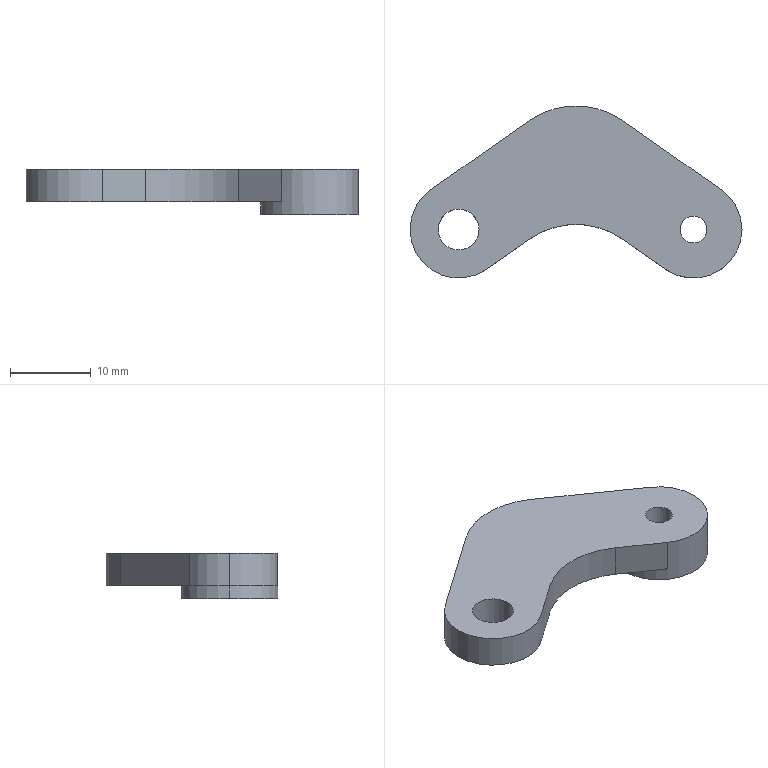Part | SolidWorks | features Attribute 3, ICE 2, Extrusion 1, Fillet 1, HoleWzd 1 | 1 solid | 17 faces | box 41 x 21.27 x 5.6 mm | volume 2205 mm3 | cylinder 10 | plane 7 | commonest cylinder face diameters 12 x4 3.3 x2 5.05 x2 20 x2
STEP:
#1=CARTESIAN_POINT('',(27.35,0.,-1.6));
#2=VERTEX_POINT('',#1);
#3=CARTESIAN_POINT('',(30.65,0.,-1.6));
#4=VERTEX_POINT('',#3);
#5=CARTESIAN_POINT('',(29.,0.,-1.6));
#6=DIRECTION('',(0.,0.,1.));
#7=DIRECTION('',(1.,0.,0.));
#8=AXIS2_PLACEMENT_3D('',#5,#6,#7);
#9=CIRCLE('',#8,1.65);
#10=EDGE_CURVE('',#2,#4,#9,.T.);
#11=ORIENTED_EDGE('',*,*,#10,.F.);
#12=CARTESIAN_POINT('',(27.35,0.,4.));
#13=VERTEX_POINT('',#12);
#14=CARTESIAN_POINT('',(27.35,0.,4.));
#15=DIRECTION('',(0.,0.,1.));
#16=VECTOR('',#15,1000.);
#17=LINE('',#14,#16);
#18=EDGE_CURVE('',#2,#13,#17,.T.);
#19=ORIENTED_EDGE('',*,*,#18,.T.);
#20=CARTESIAN_POINT('',(30.65,0.,4.));
#21=VERTEX_POINT('',#20);
#22=CARTESIAN_POINT('',(29.,0.,4.));
#23=DIRECTION('',(0.,0.,1.));
#24=DIRECTION('',(1.,0.,0.));
#25=AXIS2_PLACEMENT_3D('',#22,#23,#24);
#26=CIRCLE('',#25,1.65);
#27=EDGE_CURVE('',#13,#21,#26,.T.);
#28=ORIENTED_EDGE('',*,*,#27,.T.);
#29=CARTESIAN_POINT('',(30.65,0.,4.));
#30=DIRECTION('',(0.,0.,1.));
#31=VECTOR('',#30,1000.);
#32=LINE('',#29,#31);
#33=EDGE_CURVE('',#4,#21,#32,.T.);
#34=ORIENTED_EDGE('',*,*,#33,.F.);
#35=EDGE_LOOP('',(#11,#19,#28,#34));
#36=FACE_OUTER_BOUND('',#35,.T.);
#37=CARTESIAN_POINT('',(29.,0.,4.));
#38=DIRECTION('',(0.,0.,1.));
#39=DIRECTION('',(1.,0.,0.));
#40=AXIS2_PLACEMENT_3D('',#37,#38,#39);
#41=CYLINDRICAL_SURFACE('',#40,1.65);
#42=ADVANCED_FACE('',(#36),#41,.F.);
#43=CARTESIAN_POINT('',(-2.525,0.,0.));
#44=VERTEX_POINT('',#43);
#45=CARTESIAN_POINT('',(2.525,0.,0.));
#46=VERTEX_POINT('',#45);
#47=CARTESIAN_POINT('',(0.,0.,0.));
#48=DIRECTION('',(0.,0.,1.));
#49=DIRECTION('',(1.,0.,0.));
#50=AXIS2_PLACEMENT_3D('',#47,#48,#49);
#51=CIRCLE('',#50,2.525);
#52=EDGE_CURVE('',#44,#46,#51,.T.);
#53=ORIENTED_EDGE('',*,*,#52,.F.);
#54=CARTESIAN_POINT('',(-2.525,0.,4.));
#55=VERTEX_POINT('',#54);
#56=CARTESIAN_POINT('',(-2.525,0.,-1.));
#57=DIRECTION('',(0.,0.,1.));
#58=VECTOR('',#57,1000.);
#59=LINE('',#56,#58);
#60=EDGE_CURVE('',#44,#55,#59,.T.);
#61=ORIENTED_EDGE('',*,*,#60,.T.);
#62=CARTESIAN_POINT('',(2.525,0.,4.));
#63=VERTEX_POINT('',#62);
#64=CARTESIAN_POINT('',(0.,0.,4.));
#65=DIRECTION('',(0.,0.,1.));
#66=DIRECTION('',(1.,0.,0.));
#67=AXIS2_PLACEMENT_3D('',#64,#65,#66);
#68=CIRCLE('',#67,2.525);
#69=EDGE_CURVE('',#55,#63,#68,.T.);
#70=ORIENTED_EDGE('',*,*,#69,.T.);
#71=CARTESIAN_POINT('',(2.525,0.,-1.));
#72=DIRECTION('',(0.,0.,1.));
#73=VECTOR('',#72,1000.);
#74=LINE('',#71,#73);
#75=EDGE_CURVE('',#46,#63,#74,.T.);
#76=ORIENTED_EDGE('',*,*,#75,.F.);
#77=EDGE_LOOP('',(#53,#61,#70,#76));
#78=FACE_OUTER_BOUND('',#77,.T.);
#79=CARTESIAN_POINT('',(0.,0.,-1.));
#80=DIRECTION('',(0.,0.,1.));
#81=DIRECTION('',(1.,0.,0.));
#82=AXIS2_PLACEMENT_3D('',#79,#80,#81);
#83=CYLINDRICAL_SURFACE('',#82,2.525);
#84=ADVANCED_FACE('',(#78),#83,.F.);
#85=CARTESIAN_POINT('',(35.,0.,4.));
#86=VERTEX_POINT('',#85);
#87=CARTESIAN_POINT('',(32.441,4.915,4.));
#88=VERTEX_POINT('',#87);
#89=CARTESIAN_POINT('',(29.,0.,4.));
#90=DIRECTION('',(0.,0.,1.));
#91=DIRECTION('',(1.,0.,0.));
#92=AXIS2_PLACEMENT_3D('',#89,#90,#91);
#93=CIRCLE('',#92,6.);
#94=EDGE_CURVE('',#86,#88,#93,.T.);
#95=ORIENTED_EDGE('',*,*,#94,.F.);
#96=CARTESIAN_POINT('',(35.,0.,-1.6));
#97=VERTEX_POINT('',#96);
#98=CARTESIAN_POINT('',(35.,0.,4.));
#99=DIRECTION('',(0.,0.,-1.));
#100=VECTOR('',#99,1000.);
#101=LINE('',#98,#100);
#102=EDGE_CURVE('',#86,#97,#101,.T.);
#103=ORIENTED_EDGE('',*,*,#102,.T.);
#104=CARTESIAN_POINT('',(23.,0.,-1.6));
#105=VERTEX_POINT('',#104);
#106=CARTESIAN_POINT('',(29.,0.,-1.6));
#107=DIRECTION('',(0.,0.,-1.));
#108=DIRECTION('',(-1.,0.,0.));
#109=AXIS2_PLACEMENT_3D('',#106,#107,#108);
#110=CIRCLE('',#109,6.);
#111=EDGE_CURVE('',#105,#97,#110,.T.);
#112=ORIENTED_EDGE('',*,*,#111,.F.);
#113=CARTESIAN_POINT('',(23.,0.,0.));
#114=VERTEX_POINT('',#113);
#115=CARTESIAN_POINT('',(23.,0.,4.));
#116=DIRECTION('',(0.,0.,-1.));
#117=VECTOR('',#116,1000.);
#118=LINE('',#115,#117);
#119=EDGE_CURVE('',#114,#105,#118,.T.);
#120=ORIENTED_EDGE('',*,*,#119,.F.);
#121=CARTESIAN_POINT('',(32.441,4.915,0.));
#122=VERTEX_POINT('',#121);
#123=CARTESIAN_POINT('',(29.,0.,0.));
#124=DIRECTION('',(0.,0.,-1.));
#125=DIRECTION('',(-1.,0.,0.));
#126=AXIS2_PLACEMENT_3D('',#123,#124,#125);
#127=CIRCLE('',#126,6.);
#128=EDGE_CURVE('',#114,#122,#127,.T.);
#129=ORIENTED_EDGE('',*,*,#128,.T.);
#130=CARTESIAN_POINT('',(32.441,4.915,4.));
#131=DIRECTION('',(0.,0.,-1.));
#132=VECTOR('',#131,1000.);
#133=LINE('',#130,#132);
#134=EDGE_CURVE('',#88,#122,#133,.T.);
#135=ORIENTED_EDGE('',*,*,#134,.F.);
#136=EDGE_LOOP('',(#95,#103,#112,#120,#129,#135));
#137=FACE_OUTER_BOUND('',#136,.T.);
#138=CARTESIAN_POINT('',(29.,0.,4.));
#139=DIRECTION('',(0.,0.,-1.));
#140=DIRECTION('',(-1.,0.,0.));
#141=AXIS2_PLACEMENT_3D('',#138,#139,#140);
#142=CYLINDRICAL_SURFACE('',#141,6.);
#143=ADVANCED_FACE('',(#137),#142,.T.);
#144=CARTESIAN_POINT('',(-6.,0.,4.));
#145=VERTEX_POINT('',#144);
#146=CARTESIAN_POINT('',(3.441,-4.915,4.));
#147=VERTEX_POINT('',#146);
#148=CARTESIAN_POINT('',(0.,0.,4.));
#149=DIRECTION('',(0.,0.,1.));
#150=DIRECTION('',(1.,0.,0.));
#151=AXIS2_PLACEMENT_3D('',#148,#149,#150);
#152=CIRCLE('',#151,6.);
#153=EDGE_CURVE('',#145,#147,#152,.T.);
#154=ORIENTED_EDGE('',*,*,#153,.F.);
#155=CARTESIAN_POINT('',(-6.,0.,0.));
#156=VERTEX_POINT('',#155);
#157=CARTESIAN_POINT('',(-6.,0.,4.));
#158=DIRECTION('',(0.,0.,-1.));
#159=VECTOR('',#158,1000.);
#160=LINE('',#157,#159);
#161=EDGE_CURVE('',#145,#156,#160,.T.);
#162=ORIENTED_EDGE('',*,*,#161,.T.);
#163=CARTESIAN_POINT('',(3.441,-4.915,0.));
#164=VERTEX_POINT('',#163);
#165=CARTESIAN_POINT('',(0.,0.,0.));
#166=DIRECTION('',(0.,0.,1.));
#167=DIRECTION('',(1.,0.,0.));
#168=AXIS2_PLACEMENT_3D('',#165,#166,#167);
#169=CIRCLE('',#168,6.);
#170=EDGE_CURVE('',#156,#164,#169,.T.);
#171=ORIENTED_EDGE('',*,*,#170,.T.);
#172=CARTESIAN_POINT('',(3.441,-4.915,4.));
#173=DIRECTION('',(0.,0.,-1.));
#174=VECTOR('',#173,1000.);
#175=LINE('',#172,#174);
#176=EDGE_CURVE('',#147,#164,#175,.T.);
#177=ORIENTED_EDGE('',*,*,#176,.F.);
#178=EDGE_LOOP('',(#154,#162,#171,#177));
#179=FACE_OUTER_BOUND('',#178,.T.);
#180=CARTESIAN_POINT('',(0.,0.,4.));
#181=DIRECTION('',(0.,0.,-1.));
#182=DIRECTION('',(-1.,0.,0.));
#183=AXIS2_PLACEMENT_3D('',#180,#181,#182);
#184=CYLINDRICAL_SURFACE('',#183,6.);
#185=ADVANCED_FACE('',(#179),#184,.T.);
#186=ORIENTED_EDGE('',*,*,#161,.F.);
#187=CARTESIAN_POINT('',(-3.441,4.915,4.));
#188=VERTEX_POINT('',#187);
#189=CARTESIAN_POINT('',(0.,0.,4.));
#190=DIRECTION('',(0.,0.,1.));
#191=DIRECTION('',(1.,0.,0.));
#192=AXIS2_PLACEMENT_3D('',#189,#190,#191);
#193=CIRCLE('',#192,6.);
#194=EDGE_CURVE('',#188,#145,#193,.T.);
#195=ORIENTED_EDGE('',*,*,#194,.F.);
#196=CARTESIAN_POINT('',(-3.441,4.915,0.));
#197=VERTEX_POINT('',#196);
#198=CARTESIAN_POINT('',(-3.441,4.915,4.));
#199=DIRECTION('',(0.,0.,-1.));
#200=VECTOR('',#199,1000.);
#201=LINE('',#198,#200);
#202=EDGE_CURVE('',#188,#197,#201,.T.);
#203=ORIENTED_EDGE('',*,*,#202,.T.);
#204=CARTESIAN_POINT('',(0.,0.,0.));
#205=DIRECTION('',(0.,0.,1.));
#206=DIRECTION('',(1.,0.,0.));
#207=AXIS2_PLACEMENT_3D('',#204,#205,#206);
#208=CIRCLE('',#207,6.);
#209=EDGE_CURVE('',#197,#156,#208,.T.);
#210=ORIENTED_EDGE('',*,*,#209,.T.);
#211=EDGE_LOOP('',(#186,#195,#203,#210));
#212=FACE_OUTER_BOUND('',#211,.T.);
#213=CARTESIAN_POINT('',(0.,0.,4.));
#214=DIRECTION('',(0.,0.,-1.));
#215=DIRECTION('',(-1.,0.,0.));
#216=AXIS2_PLACEMENT_3D('',#213,#214,#215);
#217=CYLINDRICAL_SURFACE('',#216,6.);
#218=ADVANCED_FACE('',(#212),#217,.T.);
#219=CARTESIAN_POINT('',(8.764,-1.188,0.));
#220=VERTEX_POINT('',#219);
#221=CARTESIAN_POINT('',(3.441,-4.915,0.));
#222=DIRECTION('',(0.8192,0.5736,0.));
#223=VECTOR('',#222,1000.);
#224=LINE('',#221,#223);
#225=EDGE_CURVE('',#164,#220,#224,.T.);
#226=ORIENTED_EDGE('',*,*,#225,.T.);
#227=CARTESIAN_POINT('',(8.764,-1.188,4.));
#228=VERTEX_POINT('',#227);
#229=CARTESIAN_POINT('',(8.764,-1.188,4.));
#230=DIRECTION('',(0.,0.,1.));
#231=VECTOR('',#230,1000.);
#232=LINE('',#229,#231);
#233=EDGE_CURVE('',#220,#228,#232,.T.);
#234=ORIENTED_EDGE('',*,*,#233,.T.);
#235=CARTESIAN_POINT('',(3.441,-4.915,4.));
#236=DIRECTION('',(0.8192,0.5736,0.));
#237=VECTOR('',#236,1000.);
#238=LINE('',#235,#237);
#239=EDGE_CURVE('',#147,#228,#238,.T.);
#240=ORIENTED_EDGE('',*,*,#239,.F.);
#241=ORIENTED_EDGE('',*,*,#176,.T.);
#242=EDGE_LOOP('',(#226,#234,#240,#241));
#243=FACE_OUTER_BOUND('',#242,.T.);
#244=CARTESIAN_POINT('',(3.441,-4.915,4.));
#245=DIRECTION('',(-0.5736,0.8192,0.));
#246=DIRECTION('',(-0.8192,-0.5736,0.));
#247=AXIS2_PLACEMENT_3D('',#244,#245,#246);
#248=PLANE('',#247);
#249=ADVANCED_FACE('',(#243),#248,.F.);
#250=CARTESIAN_POINT('',(20.236,-1.188,4.));
#251=VERTEX_POINT('',#250);
#252=CARTESIAN_POINT('',(25.559,-4.915,4.));
#253=VERTEX_POINT('',#252);
#254=CARTESIAN_POINT('',(14.5,2.828,4.));
#255=DIRECTION('',(0.8192,-0.5736,0.));
#256=VECTOR('',#255,1000.);
#257=LINE('',#254,#256);
#258=EDGE_CURVE('',#251,#253,#257,.T.);
#259=ORIENTED_EDGE('',*,*,#258,.F.);
#260=CARTESIAN_POINT('',(20.236,-1.188,0.));
#261=VERTEX_POINT('',#260);
#262=CARTESIAN_POINT('',(20.236,-1.188,0.));
#263=DIRECTION('',(0.,0.,-1.));
#264=VECTOR('',#263,1000.);
#265=LINE('',#262,#264);
#266=EDGE_CURVE('',#251,#261,#265,.T.);
#267=ORIENTED_EDGE('',*,*,#266,.T.);
#268=CARTESIAN_POINT('',(25.559,-4.915,0.));
#269=VERTEX_POINT('',#268);
#270=CARTESIAN_POINT('',(14.5,2.828,0.));
#271=DIRECTION('',(0.8192,-0.5736,0.));
#272=VECTOR('',#271,1000.);
#273=LINE('',#270,#272);
#274=EDGE_CURVE('',#261,#269,#273,.T.);
#275=ORIENTED_EDGE('',*,*,#274,.T.);
#276=CARTESIAN_POINT('',(25.559,-4.915,4.));
#277=DIRECTION('',(0.,0.,-1.));
#278=VECTOR('',#277,1000.);
#279=LINE('',#276,#278);
#280=EDGE_CURVE('',#253,#269,#279,.T.);
#281=ORIENTED_EDGE('',*,*,#280,.F.);
#282=EDGE_LOOP('',(#259,#267,#275,#281));
#283=FACE_OUTER_BOUND('',#282,.T.);
#284=CARTESIAN_POINT('',(14.5,2.828,4.));
#285=DIRECTION('',(0.5736,0.8192,0.));
#286=DIRECTION('',(-0.8192,0.5736,0.));
#287=AXIS2_PLACEMENT_3D('',#284,#285,#286);
#288=PLANE('',#287);
#289=ADVANCED_FACE('',(#283),#288,.F.);
#290=ORIENTED_EDGE('',*,*,#102,.F.);
#291=CARTESIAN_POINT('',(29.,0.,4.));
#292=DIRECTION('',(0.,0.,1.));
#293=DIRECTION('',(1.,0.,0.));
#294=AXIS2_PLACEMENT_3D('',#291,#292,#293);
#295=CIRCLE('',#294,6.);
#296=EDGE_CURVE('',#253,#86,#295,.T.);
#297=ORIENTED_EDGE('',*,*,#296,.F.);
#298=ORIENTED_EDGE('',*,*,#280,.T.);
#299=CARTESIAN_POINT('',(29.,0.,0.));
#300=DIRECTION('',(0.,0.,-1.));
#301=DIRECTION('',(-1.,0.,0.));
#302=AXIS2_PLACEMENT_3D('',#299,#300,#301);
#303=CIRCLE('',#302,6.);
#304=EDGE_CURVE('',#269,#114,#303,.T.);
#305=ORIENTED_EDGE('',*,*,#304,.T.);
#306=ORIENTED_EDGE('',*,*,#119,.T.);
#307=CARTESIAN_POINT('',(29.,0.,-1.6));
#308=DIRECTION('',(0.,0.,-1.));
#309=DIRECTION('',(-1.,0.,0.));
#310=AXIS2_PLACEMENT_3D('',#307,#308,#309);
#311=CIRCLE('',#310,6.);
#312=EDGE_CURVE('',#97,#105,#311,.T.);
#313=ORIENTED_EDGE('',*,*,#312,.F.);
#314=EDGE_LOOP('',(#290,#297,#298,#305,#306,#313));
#315=FACE_OUTER_BOUND('',#314,.T.);
#316=CARTESIAN_POINT('',(29.,0.,4.));
#317=DIRECTION('',(0.,0.,-1.));
#318=DIRECTION('',(-1.,0.,0.));
#319=AXIS2_PLACEMENT_3D('',#316,#317,#318);
#320=CYLINDRICAL_SURFACE('',#319,6.);
#321=ADVANCED_FACE('',(#315),#320,.T.);
#322=CARTESIAN_POINT('',(20.236,13.461,0.));
#323=VERTEX_POINT('',#322);
#324=CARTESIAN_POINT('',(14.5,17.478,0.));
#325=DIRECTION('',(-0.8192,0.5736,0.));
#326=VECTOR('',#325,1000.);
#327=LINE('',#324,#326);
#328=EDGE_CURVE('',#122,#323,#327,.T.);
#329=ORIENTED_EDGE('',*,*,#328,.T.);
#330=CARTESIAN_POINT('',(20.236,13.461,4.));
#331=VERTEX_POINT('',#330);
#332=CARTESIAN_POINT('',(20.236,13.461,4.));
#333=DIRECTION('',(0.,0.,1.));
#334=VECTOR('',#333,1000.);
#335=LINE('',#332,#334);
#336=EDGE_CURVE('',#323,#331,#335,.T.);
#337=ORIENTED_EDGE('',*,*,#336,.T.);
#338=CARTESIAN_POINT('',(14.5,17.478,4.));
#339=DIRECTION('',(-0.8192,0.5736,0.));
#340=VECTOR('',#339,1000.);
#341=LINE('',#338,#340);
#342=EDGE_CURVE('',#88,#331,#341,.T.);
#343=ORIENTED_EDGE('',*,*,#342,.F.);
#344=ORIENTED_EDGE('',*,*,#134,.T.);
#345=EDGE_LOOP('',(#329,#337,#343,#344));
#346=FACE_OUTER_BOUND('',#345,.T.);
#347=CARTESIAN_POINT('',(14.5,17.478,4.));
#348=DIRECTION('',(-0.5736,-0.8192,0.));
#349=DIRECTION('',(0.8192,-0.5736,0.));
#350=AXIS2_PLACEMENT_3D('',#347,#348,#349);
#351=PLANE('',#350);
#352=ADVANCED_FACE('',(#346),#351,.F.);
#353=CARTESIAN_POINT('',(8.764,13.461,4.));
#354=VERTEX_POINT('',#353);
#355=CARTESIAN_POINT('',(-3.441,4.915,4.));
#356=DIRECTION('',(-0.8192,-0.5736,0.));
#357=VECTOR('',#356,1000.);
#358=LINE('',#355,#357);
#359=EDGE_CURVE('',#354,#188,#358,.T.);
#360=ORIENTED_EDGE('',*,*,#359,.F.);
#361=CARTESIAN_POINT('',(8.764,13.461,0.));
#362=VERTEX_POINT('',#361);
#363=CARTESIAN_POINT('',(8.764,13.461,4.));
#364=DIRECTION('',(0.,0.,-1.));
#365=VECTOR('',#364,1000.);
#366=LINE('',#363,#365);
#367=EDGE_CURVE('',#354,#362,#366,.T.);
#368=ORIENTED_EDGE('',*,*,#367,.T.);
#369=CARTESIAN_POINT('',(-3.441,4.915,0.));
#370=DIRECTION('',(-0.8192,-0.5736,0.));
#371=VECTOR('',#370,1000.);
#372=LINE('',#369,#371);
#373=EDGE_CURVE('',#362,#197,#372,.T.);
#374=ORIENTED_EDGE('',*,*,#373,.T.);
#375=ORIENTED_EDGE('',*,*,#202,.F.);
#376=EDGE_LOOP('',(#360,#368,#374,#375));
#377=FACE_OUTER_BOUND('',#376,.T.);
#378=CARTESIAN_POINT('',(-3.441,4.915,4.));
#379=DIRECTION('',(0.5736,-0.8192,0.));
#380=DIRECTION('',(0.8192,0.5736,0.));
#381=AXIS2_PLACEMENT_3D('',#378,#379,#380);
#382=PLANE('',#381);
#383=ADVANCED_FACE('',(#377),#382,.F.);
#384=CARTESIAN_POINT('',(29.,0.,4.));
#385=DIRECTION('',(0.,0.,1.));
#386=DIRECTION('',(1.,0.,0.));
#387=AXIS2_PLACEMENT_3D('',#384,#385,#386);
#388=CIRCLE('',#387,1.65);
#389=EDGE_CURVE('',#21,#13,#388,.T.);
#390=ORIENTED_EDGE('',*,*,#389,.F.);
#391=ORIENTED_EDGE('',*,*,#27,.F.);
#392=EDGE_LOOP('',(#390,#391));
#393=FACE_BOUND('',#392,.T.);
#394=CARTESIAN_POINT('',(0.,0.,4.));
#395=DIRECTION('',(0.,0.,1.));
#396=DIRECTION('',(1.,0.,0.));
#397=AXIS2_PLACEMENT_3D('',#394,#395,#396);
#398=CIRCLE('',#397,2.525);
#399=EDGE_CURVE('',#63,#55,#398,.T.);
#400=ORIENTED_EDGE('',*,*,#399,.F.);
#401=ORIENTED_EDGE('',*,*,#69,.F.);
#402=EDGE_LOOP('',(#400,#401));
#403=FACE_BOUND('',#402,.T.);
#404=ORIENTED_EDGE('',*,*,#342,.T.);
#405=CARTESIAN_POINT('',(14.5,5.27,4.));
#406=DIRECTION('',(0.,0.,1.));
#407=DIRECTION('',(1.,0.,0.));
#408=AXIS2_PLACEMENT_3D('',#405,#406,#407);
#409=CIRCLE('',#408,10.);
#410=EDGE_CURVE('',#331,#354,#409,.T.);
#411=ORIENTED_EDGE('',*,*,#410,.T.);
#412=ORIENTED_EDGE('',*,*,#359,.T.);
#413=ORIENTED_EDGE('',*,*,#194,.T.);
#414=ORIENTED_EDGE('',*,*,#153,.T.);
#415=ORIENTED_EDGE('',*,*,#239,.T.);
#416=CARTESIAN_POINT('',(14.5,-9.379,4.));
#417=DIRECTION('',(0.,0.,-1.));
#418=DIRECTION('',(1.,0.,0.));
#419=AXIS2_PLACEMENT_3D('',#416,#417,#418);
#420=CIRCLE('',#419,10.);
#421=EDGE_CURVE('',#228,#251,#420,.T.);
#422=ORIENTED_EDGE('',*,*,#421,.T.);
#423=ORIENTED_EDGE('',*,*,#258,.T.);
#424=ORIENTED_EDGE('',*,*,#296,.T.);
#425=ORIENTED_EDGE('',*,*,#94,.T.);
#426=EDGE_LOOP('',(#404,#411,#412,#413,#414,#415,#422,#423,#424,#425));
#427=FACE_OUTER_BOUND('',#426,.T.);
#428=CARTESIAN_POINT('',(0.,0.,4.));
#429=DIRECTION('',(0.,0.,1.));
#430=DIRECTION('',(1.,0.,0.));
#431=AXIS2_PLACEMENT_3D('',#428,#429,#430);
#432=PLANE('',#431);
#433=ADVANCED_FACE('',(#393,#403,#427),#432,.T.);
#434=ORIENTED_EDGE('',*,*,#373,.F.);
#435=CARTESIAN_POINT('',(14.5,5.27,0.));
#436=DIRECTION('',(0.,0.,-1.));
#437=DIRECTION('',(1.,0.,0.));
#438=AXIS2_PLACEMENT_3D('',#435,#436,#437);
#439=CIRCLE('',#438,10.);
#440=EDGE_CURVE('',#362,#323,#439,.T.);
#441=ORIENTED_EDGE('',*,*,#440,.T.);
#442=ORIENTED_EDGE('',*,*,#328,.F.);
#443=ORIENTED_EDGE('',*,*,#128,.F.);
#444=ORIENTED_EDGE('',*,*,#304,.F.);
#445=ORIENTED_EDGE('',*,*,#274,.F.);
#446=CARTESIAN_POINT('',(14.5,-9.379,0.));
#447=DIRECTION('',(0.,0.,1.));
#448=DIRECTION('',(1.,0.,0.));
#449=AXIS2_PLACEMENT_3D('',#446,#447,#448);
#450=CIRCLE('',#449,10.);
#451=EDGE_CURVE('',#261,#220,#450,.T.);
#452=ORIENTED_EDGE('',*,*,#451,.T.);
#453=ORIENTED_EDGE('',*,*,#225,.F.);
#454=ORIENTED_EDGE('',*,*,#170,.F.);
#455=ORIENTED_EDGE('',*,*,#209,.F.);
#456=EDGE_LOOP('',(#434,#441,#442,#443,#444,#445,#452,#453,#454,#455));
#457=FACE_OUTER_BOUND('',#456,.T.);
#458=CARTESIAN_POINT('',(0.,0.,0.));
#459=DIRECTION('',(0.,0.,1.));
#460=DIRECTION('',(1.,0.,0.));
#461=AXIS2_PLACEMENT_3D('',#458,#459,#460);
#462=CIRCLE('',#461,2.525);
#463=EDGE_CURVE('',#46,#44,#462,.T.);
#464=ORIENTED_EDGE('',*,*,#463,.T.);
#465=ORIENTED_EDGE('',*,*,#52,.T.);
#466=EDGE_LOOP('',(#464,#465));
#467=FACE_BOUND('',#466,.T.);
#468=CARTESIAN_POINT('',(0.,0.,0.));
#469=DIRECTION('',(0.,0.,1.));
#470=DIRECTION('',(1.,0.,0.));
#471=AXIS2_PLACEMENT_3D('',#468,#469,#470);
#472=PLANE('',#471);
#473=ADVANCED_FACE('',(#457,#467),#472,.F.);
#474=ORIENTED_EDGE('',*,*,#60,.F.);
#475=ORIENTED_EDGE('',*,*,#463,.F.);
#476=ORIENTED_EDGE('',*,*,#75,.T.);
#477=ORIENTED_EDGE('',*,*,#399,.T.);
#478=EDGE_LOOP('',(#474,#475,#476,#477));
#479=FACE_OUTER_BOUND('',#478,.T.);
#480=CARTESIAN_POINT('',(0.,0.,-1.));
#481=DIRECTION('',(0.,0.,1.));
#482=DIRECTION('',(1.,0.,0.));
#483=AXIS2_PLACEMENT_3D('',#480,#481,#482);
#484=CYLINDRICAL_SURFACE('',#483,2.525);
#485=ADVANCED_FACE('',(#479),#484,.F.);
#486=CARTESIAN_POINT('',(29.,0.,-1.6));
#487=DIRECTION('',(0.,0.,1.));
#488=DIRECTION('',(1.,0.,0.));
#489=AXIS2_PLACEMENT_3D('',#486,#487,#488);
#490=CIRCLE('',#489,1.65);
#491=EDGE_CURVE('',#4,#2,#490,.T.);
#492=ORIENTED_EDGE('',*,*,#491,.T.);
#493=ORIENTED_EDGE('',*,*,#10,.T.);
#494=EDGE_LOOP('',(#492,#493));
#495=FACE_BOUND('',#494,.T.);
#496=ORIENTED_EDGE('',*,*,#111,.T.);
#497=ORIENTED_EDGE('',*,*,#312,.T.);
#498=EDGE_LOOP('',(#496,#497));
#499=FACE_OUTER_BOUND('',#498,.T.);
#500=CARTESIAN_POINT('',(29.,0.,-1.6));
#501=DIRECTION('',(0.,0.,-1.));
#502=DIRECTION('',(-1.,0.,0.));
#503=AXIS2_PLACEMENT_3D('',#500,#501,#502);
#504=PLANE('',#503);
#505=ADVANCED_FACE('',(#495,#499),#504,.T.);
#506=ORIENTED_EDGE('',*,*,#18,.F.);
#507=ORIENTED_EDGE('',*,*,#491,.F.);
#508=ORIENTED_EDGE('',*,*,#33,.T.);
#509=ORIENTED_EDGE('',*,*,#389,.T.);
#510=EDGE_LOOP('',(#506,#507,#508,#509));
#511=FACE_OUTER_BOUND('',#510,.T.);
#512=CARTESIAN_POINT('',(29.,0.,4.));
#513=DIRECTION('',(0.,0.,1.));
#514=DIRECTION('',(1.,0.,0.));
#515=AXIS2_PLACEMENT_3D('',#512,#513,#514);
#516=CYLINDRICAL_SURFACE('',#515,1.65);
#517=ADVANCED_FACE('',(#511),#516,.F.);
#518=ORIENTED_EDGE('',*,*,#410,.F.);
#519=ORIENTED_EDGE('',*,*,#336,.F.);
#520=ORIENTED_EDGE('',*,*,#440,.F.);
#521=ORIENTED_EDGE('',*,*,#367,.F.);
#522=EDGE_LOOP('',(#518,#519,#520,#521));
#523=FACE_OUTER_BOUND('',#522,.T.);
#524=CARTESIAN_POINT('',(14.5,5.27,4.));
#525=DIRECTION('',(0.,0.,-1.));
#526=DIRECTION('',(-1.,0.,0.));
#527=AXIS2_PLACEMENT_3D('',#524,#525,#526);
#528=CYLINDRICAL_SURFACE('',#527,10.);
#529=ADVANCED_FACE('',(#523),#528,.T.);
#530=ORIENTED_EDGE('',*,*,#421,.F.);
#531=ORIENTED_EDGE('',*,*,#233,.F.);
#532=ORIENTED_EDGE('',*,*,#451,.F.);
#533=ORIENTED_EDGE('',*,*,#266,.F.);
#534=EDGE_LOOP('',(#530,#531,#532,#533));
#535=FACE_OUTER_BOUND('',#534,.T.);
#536=CARTESIAN_POINT('',(14.5,-9.379,4.));
#537=DIRECTION('',(0.,0.,1.));
#538=DIRECTION('',(1.,0.,0.));
#539=AXIS2_PLACEMENT_3D('',#536,#537,#538);
#540=CYLINDRICAL_SURFACE('',#539,10.);
#541=ADVANCED_FACE('',(#535),#540,.F.);
#542=CLOSED_SHELL('',(#42,#84,#143,#185,#218,#249,#289,#321,#352,#383,#433,#473,#485,#505,#517,#529,#541));
#543=MANIFOLD_SOLID_BREP('',#542);
#544=CARTESIAN_POINT('',(0.,0.,0.));
#545=DIRECTION('',(0.,0.,1.));
#546=DIRECTION('',(1.,0.,0.));
#547=AXIS2_PLACEMENT_3D('',#544,#545,#546);
#548=(LENGTH_UNIT()NAMED_UNIT(*)SI_UNIT(.MILLI.,.METRE.));
#549=UNCERTAINTY_MEASURE_WITH_UNIT(LENGTH_MEASURE(0.00001),#548,'','');
#550=(NAMED_UNIT(*)PLANE_ANGLE_UNIT()SI_UNIT($,.RADIAN.));
#551=(NAMED_UNIT(*)SI_UNIT($,.STERADIAN.)SOLID_ANGLE_UNIT());
#552=(GEOMETRIC_REPRESENTATION_CONTEXT(3)GLOBAL_UNCERTAINTY_ASSIGNED_CONTEXT((#549))GLOBAL_UNIT_ASSIGNED_CONTEXT((#548,#550,#551))REPRESENTATION_CONTEXT('',''));
#553=ADVANCED_BREP_SHAPE_REPRESENTATION('',(#543,#547),#552);